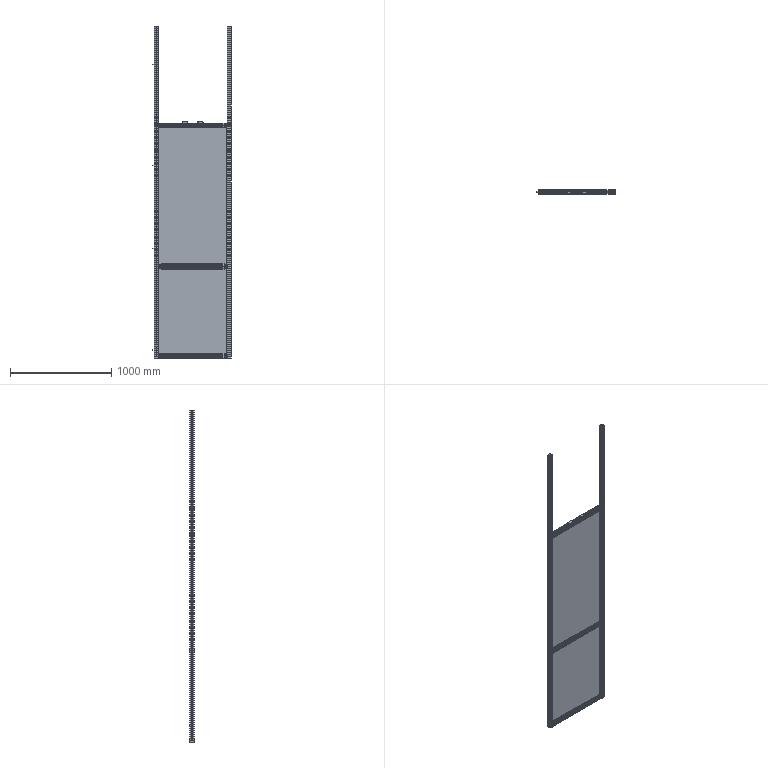Part | SolidWorks | features ReferencePattern 21, LocalLPattern 5, CompositeCurve 2 | 49 solids | 2264 faces | box 772.4 x 40 x 3280 mm | volume 13403212 mm3 | plane 1495 | cylinder 649 | cone 108 | spline 12 | commonest cylinder face diameters 6.8 x127 2 x54 19 x36 6.6 x32 11 x32 20.854 x32